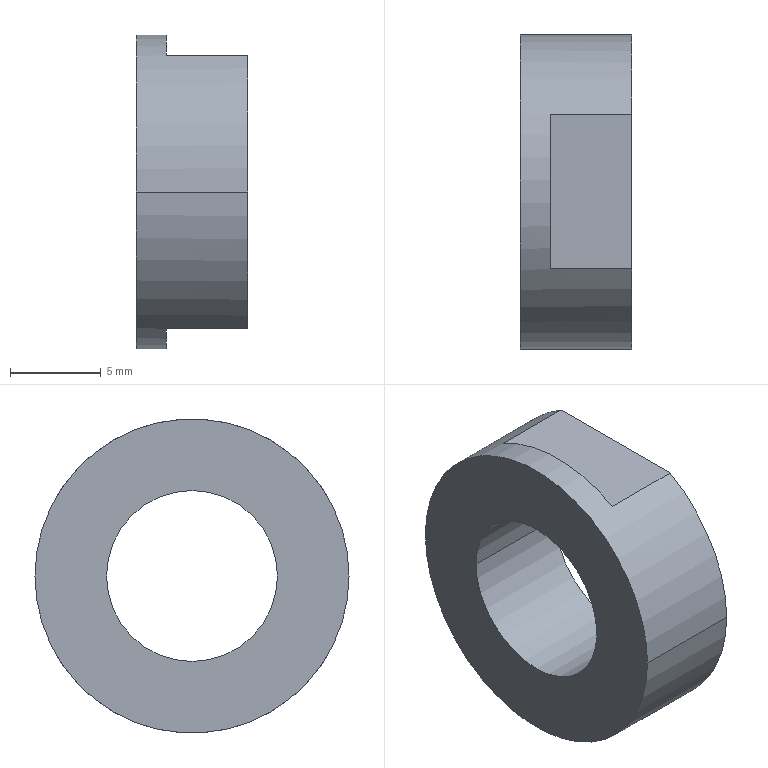Part | STEP file | BREP_4 | 1 solid | 10 faces | box 6.16 x 17.28 x 17.28 mm | volume 959.564 mm3 | plane 6 | cylinder 4 | commonest cylinder face diameters 9.4 x2 17.28 x2
STEP:
#1=CARTESIAN_POINT('',(0.,0.,0.));
#2=DIRECTION('',(0.,0.,1.));
#3=DIRECTION('',(1.,0.,0.));
#4=AXIS2_PLACEMENT_3D('',#1,#2,#3);
#5=CARTESIAN_POINT('',(56.72,-8.64,0.));
#6=VERTEX_POINT('',#5);
#7=CARTESIAN_POINT('',(56.72,8.64,0.));
#8=VERTEX_POINT('',#7);
#9=CARTESIAN_POINT('',(56.72,0.,0.));
#10=DIRECTION('',(-1.,0.,0.));
#11=DIRECTION('',(0.,-1.,0.));
#12=AXIS2_PLACEMENT_3D('',#9,#10,#11);
#13=CIRCLE('',#12,8.64);
#14=CARTESIAN_POINT('',(56.72,-8.64,8.64));
#15=DIRECTION('',(-1.,0.,0.));
#16=DIRECTION('',(0.,1.,0.));
#17=AXIS2_PLACEMENT_3D('',#14,#15,#16);
#18=PLANE('',#17);
#19=CARTESIAN_POINT('',(8.64,8.64));
#20=DIRECTION('',(-1.,0.));
#21=AXIS2_PLACEMENT_2D('',#19,#20);
#22=CIRCLE('',#21,8.64);
#23=(GEOMETRIC_REPRESENTATION_CONTEXT(2)PARAMETRIC_REPRESENTATION_CONTEXT()REPRESENTATION_CONTEXT('',''));
#24=DEFINITIONAL_REPRESENTATION('',(#22),#23);
#25=PCURVE('',#18,#24);
#26=CARTESIAN_POINT('',(59.8,0.,0.));
#27=DIRECTION('',(1.,0.,0.));
#28=DIRECTION('',(0.,1.,0.));
#29=AXIS2_PLACEMENT_3D('',#26,#27,#28);
#30=CYLINDRICAL_SURFACE('',#29,8.64);
#31=CARTESIAN_POINT('',(3.142,-3.08));
#32=DIRECTION('',(-1.,0.));
#33=VECTOR('',#32,1.);
#34=LINE('',#31,#33);
#35=(GEOMETRIC_REPRESENTATION_CONTEXT(2)PARAMETRIC_REPRESENTATION_CONTEXT()REPRESENTATION_CONTEXT('',''));
#36=DEFINITIONAL_REPRESENTATION('',(#34),#35);
#37=PCURVE('',#30,#36);
#38=SURFACE_CURVE('',#13,(#25,#37),.PCURVE_S1.);
#39=EDGE_CURVE('',#6,#8,#38,.T.);
#40=ORIENTED_EDGE('',*,*,#39,.F.);
#41=CARTESIAN_POINT('',(56.72,0.,0.));
#42=DIRECTION('',(-1.,0.,0.));
#43=DIRECTION('',(0.,1.,0.));
#44=AXIS2_PLACEMENT_3D('',#41,#42,#43);
#45=CIRCLE('',#44,8.64);
#46=CARTESIAN_POINT('',(8.64,8.64));
#47=DIRECTION('',(1.,0.));
#48=AXIS2_PLACEMENT_2D('',#46,#47);
#49=CIRCLE('',#48,8.64);
#50=(GEOMETRIC_REPRESENTATION_CONTEXT(2)PARAMETRIC_REPRESENTATION_CONTEXT()REPRESENTATION_CONTEXT('',''));
#51=DEFINITIONAL_REPRESENTATION('',(#49),#50);
#52=PCURVE('',#18,#51);
#53=CARTESIAN_POINT('',(59.8,0.,0.));
#54=DIRECTION('',(1.,0.,0.));
#55=DIRECTION('',(0.,-1.,0.));
#56=AXIS2_PLACEMENT_3D('',#53,#54,#55);
#57=CYLINDRICAL_SURFACE('',#56,8.64);
#58=CARTESIAN_POINT('',(3.142,-3.08));
#59=DIRECTION('',(-1.,0.));
#60=VECTOR('',#59,1.);
#61=LINE('',#58,#60);
#62=(GEOMETRIC_REPRESENTATION_CONTEXT(2)PARAMETRIC_REPRESENTATION_CONTEXT()REPRESENTATION_CONTEXT('',''));
#63=DEFINITIONAL_REPRESENTATION('',(#61),#62);
#64=PCURVE('',#57,#63);
#65=SURFACE_CURVE('',#45,(#52,#64),.PCURVE_S1.);
#66=EDGE_CURVE('',#8,#6,#65,.T.);
#67=ORIENTED_EDGE('',*,*,#66,.F.);
#68=EDGE_LOOP('',(#40,#67));
#69=FACE_BOUND('',#68,.F.);
#70=CARTESIAN_POINT('',(56.72,4.7,0.));
#71=VERTEX_POINT('',#70);
#72=CARTESIAN_POINT('',(56.72,-4.7,0.));
#73=VERTEX_POINT('',#72);
#74=CARTESIAN_POINT('',(56.72,0.,0.));
#75=DIRECTION('',(1.,0.,0.));
#76=DIRECTION('',(0.,1.,0.));
#77=AXIS2_PLACEMENT_3D('',#74,#75,#76);
#78=CIRCLE('',#77,4.7);
#79=CARTESIAN_POINT('',(13.34,8.64));
#80=CARTESIAN_POINT('',(13.34,0.4994));
#81=CARTESIAN_POINT('',(6.29,4.57));
#82=CARTESIAN_POINT('',(-0.76,8.64));
#83=CARTESIAN_POINT('',(6.29,12.71));
#84=CARTESIAN_POINT('',(13.34,16.781));
#85=CARTESIAN_POINT('',(13.34,8.64));
#86=(BOUNDED_CURVE()B_SPLINE_CURVE(2,(#79,#80,#81,#82,#83,#84,#85),.UNSPECIFIED.,.T.,.F.)B_SPLINE_CURVE_WITH_KNOTS((1,2,2,2,2,1),(-2.094,0.,2.094,4.189,6.283,8.378),.UNSPECIFIED.)CURVE()GEOMETRIC_REPRESENTATION_ITEM()RATIONAL_B_SPLINE_CURVE((1.,0.5,1.,0.5,1.,0.5,1.))REPRESENTATION_ITEM(''));
#87=(GEOMETRIC_REPRESENTATION_CONTEXT(2)PARAMETRIC_REPRESENTATION_CONTEXT()REPRESENTATION_CONTEXT('',''));
#88=DEFINITIONAL_REPRESENTATION('',(#86),#87);
#89=PCURVE('',#18,#88);
#90=CARTESIAN_POINT('',(59.8,0.,0.));
#91=DIRECTION('',(1.,0.,0.));
#92=DIRECTION('',(0.,-1.,0.));
#93=AXIS2_PLACEMENT_3D('',#90,#91,#92);
#94=CYLINDRICAL_SURFACE('',#93,4.7);
#95=CARTESIAN_POINT('',(3.142,-3.08));
#96=DIRECTION('',(1.,0.));
#97=VECTOR('',#96,1.);
#98=LINE('',#95,#97);
#99=(GEOMETRIC_REPRESENTATION_CONTEXT(2)PARAMETRIC_REPRESENTATION_CONTEXT()REPRESENTATION_CONTEXT('',''));
#100=DEFINITIONAL_REPRESENTATION('',(#98),#99);
#101=PCURVE('',#94,#100);
#102=SURFACE_CURVE('',#78,(#89,#101),.PCURVE_S1.);
#103=EDGE_CURVE('',#71,#73,#102,.T.);
#104=ORIENTED_EDGE('',*,*,#103,.F.);
#105=CARTESIAN_POINT('',(56.72,0.,0.));
#106=DIRECTION('',(1.,0.,0.));
#107=DIRECTION('',(0.,-1.,0.));
#108=AXIS2_PLACEMENT_3D('',#105,#106,#107);
#109=CIRCLE('',#108,4.7);
#110=CARTESIAN_POINT('',(3.94,8.64));
#111=CARTESIAN_POINT('',(3.94,16.781));
#112=CARTESIAN_POINT('',(10.99,12.71));
#113=CARTESIAN_POINT('',(18.04,8.64));
#114=CARTESIAN_POINT('',(10.99,4.57));
#115=CARTESIAN_POINT('',(3.94,0.4994));
#116=CARTESIAN_POINT('',(3.94,8.64));
#117=(BOUNDED_CURVE()B_SPLINE_CURVE(2,(#110,#111,#112,#113,#114,#115,#116),.UNSPECIFIED.,.T.,.F.)B_SPLINE_CURVE_WITH_KNOTS((1,2,2,2,2,1),(-2.094,0.,2.094,4.189,6.283,8.378),.UNSPECIFIED.)CURVE()GEOMETRIC_REPRESENTATION_ITEM()RATIONAL_B_SPLINE_CURVE((1.,0.5,1.,0.5,1.,0.5,1.))REPRESENTATION_ITEM(''));
#118=(GEOMETRIC_REPRESENTATION_CONTEXT(2)PARAMETRIC_REPRESENTATION_CONTEXT()REPRESENTATION_CONTEXT('',''));
#119=DEFINITIONAL_REPRESENTATION('',(#117),#118);
#120=PCURVE('',#18,#119);
#121=CARTESIAN_POINT('',(59.8,0.,0.));
#122=DIRECTION('',(1.,0.,0.));
#123=DIRECTION('',(0.,1.,0.));
#124=AXIS2_PLACEMENT_3D('',#121,#122,#123);
#125=CYLINDRICAL_SURFACE('',#124,4.7);
#126=CARTESIAN_POINT('',(3.142,-3.08));
#127=DIRECTION('',(1.,0.));
#128=VECTOR('',#127,1.);
#129=LINE('',#126,#128);
#130=(GEOMETRIC_REPRESENTATION_CONTEXT(2)PARAMETRIC_REPRESENTATION_CONTEXT()REPRESENTATION_CONTEXT('',''));
#131=DEFINITIONAL_REPRESENTATION('',(#129),#130);
#132=PCURVE('',#125,#131);
#133=SURFACE_CURVE('',#109,(#120,#132),.PCURVE_S1.);
#134=EDGE_CURVE('',#73,#71,#133,.T.);
#135=ORIENTED_EDGE('',*,*,#134,.F.);
#136=EDGE_LOOP('',(#104,#135));
#137=FACE_BOUND('',#136,.F.);
#138=ADVANCED_FACE('',(#69,#137),#18,.T.);
#139=CARTESIAN_POINT('',(62.88,-8.64,0.));
#140=VERTEX_POINT('',#139);
#141=CARTESIAN_POINT('',(62.88,-8.64,0.));
#142=DIRECTION('',(-1.,0.,0.));
#143=VECTOR('',#142,1.);
#144=LINE('',#141,#143);
#145=CARTESIAN_POINT('',(3.142,3.08));
#146=DIRECTION('',(0.,-1.));
#147=VECTOR('',#146,1.);
#148=LINE('',#145,#147);
#149=(GEOMETRIC_REPRESENTATION_CONTEXT(2)PARAMETRIC_REPRESENTATION_CONTEXT()REPRESENTATION_CONTEXT('',''));
#150=DEFINITIONAL_REPRESENTATION('',(#148),#149);
#151=PCURVE('',#30,#150);
#152=CARTESIAN_POINT('',(0.,3.08));
#153=DIRECTION('',(0.,-1.));
#154=VECTOR('',#153,1.);
#155=LINE('',#152,#154);
#156=(GEOMETRIC_REPRESENTATION_CONTEXT(2)PARAMETRIC_REPRESENTATION_CONTEXT()REPRESENTATION_CONTEXT('',''));
#157=DEFINITIONAL_REPRESENTATION('',(#155),#156);
#158=PCURVE('',#57,#157);
#159=SURFACE_CURVE('',#144,(#151,#158),.PCURVE_S1.);
#160=EDGE_CURVE('',#140,#6,#159,.T.);
#161=ORIENTED_EDGE('',*,*,#160,.F.);
#162=CARTESIAN_POINT('',(62.88,-4.245,7.525));
#163=VERTEX_POINT('',#162);
#164=CARTESIAN_POINT('',(62.88,0.,0.));
#165=DIRECTION('',(1.,0.,0.));
#166=DIRECTION('',(0.,-0.4914,0.8709));
#167=AXIS2_PLACEMENT_3D('',#164,#165,#166);
#168=CIRCLE('',#167,8.64);
#169=CARTESIAN_POINT('',(2.084,3.08));
#170=DIRECTION('',(1.,0.));
#171=VECTOR('',#170,1.);
#172=LINE('',#169,#171);
#173=(GEOMETRIC_REPRESENTATION_CONTEXT(2)PARAMETRIC_REPRESENTATION_CONTEXT()REPRESENTATION_CONTEXT('',''));
#174=DEFINITIONAL_REPRESENTATION('',(#172),#173);
#175=PCURVE('',#30,#174);
#176=CARTESIAN_POINT('',(62.88,-8.64,7.525));
#177=DIRECTION('',(1.,0.,0.));
#178=DIRECTION('',(0.,1.,0.));
#179=AXIS2_PLACEMENT_3D('',#176,#177,#178);
#180=PLANE('',#179);
#181=CARTESIAN_POINT('',(8.64,-7.525));
#182=DIRECTION('',(-0.4914,0.8709));
#183=AXIS2_PLACEMENT_2D('',#181,#182);
#184=CIRCLE('',#183,8.64);
#185=(GEOMETRIC_REPRESENTATION_CONTEXT(2)PARAMETRIC_REPRESENTATION_CONTEXT()REPRESENTATION_CONTEXT('',''));
#186=DEFINITIONAL_REPRESENTATION('',(#184),#185);
#187=PCURVE('',#180,#186);
#188=SURFACE_CURVE('',#168,(#175,#187),.PCURVE_S1.);
#189=EDGE_CURVE('',#163,#140,#188,.T.);
#190=ORIENTED_EDGE('',*,*,#189,.F.);
#191=CARTESIAN_POINT('',(58.38,-4.245,7.525));
#192=VERTEX_POINT('',#191);
#193=CARTESIAN_POINT('',(62.88,-4.245,7.525));
#194=DIRECTION('',(-1.,0.,0.));
#195=VECTOR('',#194,1.);
#196=LINE('',#193,#195);
#197=CARTESIAN_POINT('',(2.084,3.08));
#198=DIRECTION('',(0.,-1.));
#199=VECTOR('',#198,1.);
#200=LINE('',#197,#199);
#201=(GEOMETRIC_REPRESENTATION_CONTEXT(2)PARAMETRIC_REPRESENTATION_CONTEXT()REPRESENTATION_CONTEXT('',''));
#202=DEFINITIONAL_REPRESENTATION('',(#200),#201);
#203=PCURVE('',#30,#202);
#204=CARTESIAN_POINT('',(62.88,-4.245,7.525));
#205=DIRECTION('',(0.,0.,1.));
#206=DIRECTION('',(1.,0.,0.));
#207=AXIS2_PLACEMENT_3D('',#204,#205,#206);
#208=PLANE('',#207);
#209=CARTESIAN_POINT('',(0.,-0.000002642));
#210=DIRECTION('',(-1.,0.));
#211=VECTOR('',#210,1.);
#212=LINE('',#209,#211);
#213=(GEOMETRIC_REPRESENTATION_CONTEXT(2)PARAMETRIC_REPRESENTATION_CONTEXT()REPRESENTATION_CONTEXT('',''));
#214=DEFINITIONAL_REPRESENTATION('',(#212),#213);
#215=PCURVE('',#208,#214);
#216=SURFACE_CURVE('',#196,(#203,#215),.PCURVE_S1.);
#217=EDGE_CURVE('',#163,#192,#216,.T.);
#218=ORIENTED_EDGE('',*,*,#217,.T.);
#219=CARTESIAN_POINT('',(58.38,4.245,7.525));
#220=VERTEX_POINT('',#219);
#221=CARTESIAN_POINT('',(58.38,0.,0.));
#222=DIRECTION('',(1.,0.,0.));
#223=DIRECTION('',(0.,0.4914,0.8709));
#224=AXIS2_PLACEMENT_3D('',#221,#222,#223);
#225=CIRCLE('',#224,8.64);
#226=CARTESIAN_POINT('',(1.057,-1.42));
#227=DIRECTION('',(1.,0.));
#228=VECTOR('',#227,1.);
#229=LINE('',#226,#228);
#230=(GEOMETRIC_REPRESENTATION_CONTEXT(2)PARAMETRIC_REPRESENTATION_CONTEXT()REPRESENTATION_CONTEXT('',''));
#231=DEFINITIONAL_REPRESENTATION('',(#229),#230);
#232=PCURVE('',#30,#231);
#233=CARTESIAN_POINT('',(58.38,-4.245,8.651));
#234=DIRECTION('',(1.,0.,0.));
#235=DIRECTION('',(0.,1.,0.));
#236=AXIS2_PLACEMENT_3D('',#233,#234,#235);
#237=PLANE('',#236);
#238=CARTESIAN_POINT('',(4.245,-8.651));
#239=DIRECTION('',(0.4914,0.8709));
#240=AXIS2_PLACEMENT_2D('',#238,#239);
#241=CIRCLE('',#240,8.64);
#242=(GEOMETRIC_REPRESENTATION_CONTEXT(2)PARAMETRIC_REPRESENTATION_CONTEXT()REPRESENTATION_CONTEXT('',''));
#243=DEFINITIONAL_REPRESENTATION('',(#241),#242);
#244=PCURVE('',#237,#243);
#245=SURFACE_CURVE('',#225,(#232,#244),.PCURVE_S1.);
#246=EDGE_CURVE('',#220,#192,#245,.T.);
#247=ORIENTED_EDGE('',*,*,#246,.F.);
#248=CARTESIAN_POINT('',(62.88,4.245,7.525));
#249=VERTEX_POINT('',#248);
#250=CARTESIAN_POINT('',(58.38,4.245,7.525));
#251=DIRECTION('',(1.,0.,0.));
#252=VECTOR('',#251,1.);
#253=LINE('',#250,#252);
#254=CARTESIAN_POINT('',(1.057,-1.42));
#255=DIRECTION('',(0.,1.));
#256=VECTOR('',#255,1.);
#257=LINE('',#254,#256);
#258=(GEOMETRIC_REPRESENTATION_CONTEXT(2)PARAMETRIC_REPRESENTATION_CONTEXT()REPRESENTATION_CONTEXT('',''));
#259=DEFINITIONAL_REPRESENTATION('',(#257),#258);
#260=PCURVE('',#30,#259);
#261=CARTESIAN_POINT('',(-4.5,8.491));
#262=DIRECTION('',(1.,0.));
#263=VECTOR('',#262,1.);
#264=LINE('',#261,#263);
#265=(GEOMETRIC_REPRESENTATION_CONTEXT(2)PARAMETRIC_REPRESENTATION_CONTEXT()REPRESENTATION_CONTEXT('',''));
#266=DEFINITIONAL_REPRESENTATION('',(#264),#265);
#267=PCURVE('',#208,#266);
#268=SURFACE_CURVE('',#253,(#260,#267),.PCURVE_S1.);
#269=EDGE_CURVE('',#220,#249,#268,.T.);
#270=ORIENTED_EDGE('',*,*,#269,.T.);
#271=CARTESIAN_POINT('',(62.88,8.64,0.));
#272=VERTEX_POINT('',#271);
#273=CARTESIAN_POINT('',(62.88,0.,0.));
#274=DIRECTION('',(1.,0.,0.));
#275=DIRECTION('',(0.,1.,0.));
#276=AXIS2_PLACEMENT_3D('',#273,#274,#275);
#277=CIRCLE('',#276,8.64);
#278=CARTESIAN_POINT('',(0.,3.08));
#279=DIRECTION('',(1.,0.));
#280=VECTOR('',#279,1.);
#281=LINE('',#278,#280);
#282=(GEOMETRIC_REPRESENTATION_CONTEXT(2)PARAMETRIC_REPRESENTATION_CONTEXT()REPRESENTATION_CONTEXT('',''));
#283=DEFINITIONAL_REPRESENTATION('',(#281),#282);
#284=PCURVE('',#30,#283);
#285=CARTESIAN_POINT('',(8.64,-7.525));
#286=DIRECTION('',(1.,0.));
#287=AXIS2_PLACEMENT_2D('',#285,#286);
#288=CIRCLE('',#287,8.64);
#289=(GEOMETRIC_REPRESENTATION_CONTEXT(2)PARAMETRIC_REPRESENTATION_CONTEXT()REPRESENTATION_CONTEXT('',''));
#290=DEFINITIONAL_REPRESENTATION('',(#288),#289);
#291=PCURVE('',#180,#290);
#292=SURFACE_CURVE('',#277,(#284,#291),.PCURVE_S1.);
#293=EDGE_CURVE('',#272,#249,#292,.T.);
#294=ORIENTED_EDGE('',*,*,#293,.F.);
#295=CARTESIAN_POINT('',(62.88,8.64,0.));
#296=DIRECTION('',(-1.,0.,0.));
#297=VECTOR('',#296,1.);
#298=LINE('',#295,#297);
#299=CARTESIAN_POINT('',(0.,3.08));
#300=DIRECTION('',(0.,-1.));
#301=VECTOR('',#300,1.);
#302=LINE('',#299,#301);
#303=(GEOMETRIC_REPRESENTATION_CONTEXT(2)PARAMETRIC_REPRESENTATION_CONTEXT()REPRESENTATION_CONTEXT('',''));
#304=DEFINITIONAL_REPRESENTATION('',(#302),#303);
#305=PCURVE('',#30,#304);
#306=CARTESIAN_POINT('',(3.142,3.08));
#307=DIRECTION('',(0.,-1.));
#308=VECTOR('',#307,1.);
#309=LINE('',#306,#308);
#310=(GEOMETRIC_REPRESENTATION_CONTEXT(2)PARAMETRIC_REPRESENTATION_CONTEXT()REPRESENTATION_CONTEXT('',''));
#311=DEFINITIONAL_REPRESENTATION('',(#309),#310);
#312=PCURVE('',#57,#311);
#313=SURFACE_CURVE('',#298,(#305,#312),.PCURVE_S1.);
#314=EDGE_CURVE('',#272,#8,#313,.T.);
#315=ORIENTED_EDGE('',*,*,#314,.T.);
#316=ORIENTED_EDGE('',*,*,#39,.F.);
#317=EDGE_LOOP('',(#161,#190,#218,#247,#270,#294,#315,#316));
#318=FACE_BOUND('',#317,.T.);
#319=ADVANCED_FACE('',(#318),#30,.T.);
#320=CARTESIAN_POINT('',(62.88,4.245,-7.525));
#321=VERTEX_POINT('',#320);
#322=CARTESIAN_POINT('',(62.88,0.,0.));
#323=DIRECTION('',(1.,0.,0.));
#324=DIRECTION('',(0.,0.4914,-0.8709));
#325=AXIS2_PLACEMENT_3D('',#322,#323,#324);
#326=CIRCLE('',#325,8.64);
#327=CARTESIAN_POINT('',(2.084,3.08));
#328=DIRECTION('',(1.,0.));
#329=VECTOR('',#328,1.);
#330=LINE('',#327,#329);
#331=(GEOMETRIC_REPRESENTATION_CONTEXT(2)PARAMETRIC_REPRESENTATION_CONTEXT()REPRESENTATION_CONTEXT('',''));
#332=DEFINITIONAL_REPRESENTATION('',(#330),#331);
#333=PCURVE('',#57,#332);
#334=CARTESIAN_POINT('',(8.64,-7.525));
#335=DIRECTION('',(0.4914,-0.8709));
#336=AXIS2_PLACEMENT_2D('',#334,#335);
#337=CIRCLE('',#336,8.64);
#338=(GEOMETRIC_REPRESENTATION_CONTEXT(2)PARAMETRIC_REPRESENTATION_CONTEXT()REPRESENTATION_CONTEXT('',''));
#339=DEFINITIONAL_REPRESENTATION('',(#337),#338);
#340=PCURVE('',#180,#339);
#341=SURFACE_CURVE('',#326,(#333,#340),.PCURVE_S1.);
#342=EDGE_CURVE('',#321,#272,#341,.T.);
#343=ORIENTED_EDGE('',*,*,#342,.F.);
#344=CARTESIAN_POINT('',(58.38,4.245,-7.525));
#345=VERTEX_POINT('',#344);
#346=CARTESIAN_POINT('',(62.88,4.245,-7.525));
#347=DIRECTION('',(-1.,0.,0.));
#348=VECTOR('',#347,1.);
#349=LINE('',#346,#348);
#350=CARTESIAN_POINT('',(2.084,3.08));
#351=DIRECTION('',(0.,-1.));
#352=VECTOR('',#351,1.);
#353=LINE('',#350,#352);
#354=(GEOMETRIC_REPRESENTATION_CONTEXT(2)PARAMETRIC_REPRESENTATION_CONTEXT()REPRESENTATION_CONTEXT('',''));
#355=DEFINITIONAL_REPRESENTATION('',(#353),#354);
#356=PCURVE('',#57,#355);
#357=CARTESIAN_POINT('',(62.88,4.245,-7.525));
#358=DIRECTION('',(0.,0.,-1.));
#359=DIRECTION('',(1.,0.,0.));
#360=AXIS2_PLACEMENT_3D('',#357,#358,#359);
#361=PLANE('',#360);
#362=CARTESIAN_POINT('',(0.,-0.000002642));
#363=DIRECTION('',(-1.,0.));
#364=VECTOR('',#363,1.);
#365=LINE('',#362,#364);
#366=(GEOMETRIC_REPRESENTATION_CONTEXT(2)PARAMETRIC_REPRESENTATION_CONTEXT()REPRESENTATION_CONTEXT('',''));
#367=DEFINITIONAL_REPRESENTATION('',(#365),#366);
#368=PCURVE('',#361,#367);
#369=SURFACE_CURVE('',#349,(#356,#368),.PCURVE_S1.);
#370=EDGE_CURVE('',#321,#345,#369,.T.);
#371=ORIENTED_EDGE('',*,*,#370,.T.);
#372=CARTESIAN_POINT('',(58.38,-4.245,-7.525));
#373=VERTEX_POINT('',#372);
#374=CARTESIAN_POINT('',(58.38,0.,0.));
#375=DIRECTION('',(1.,0.,0.));
#376=DIRECTION('',(0.,-0.4914,-0.8709));
#377=AXIS2_PLACEMENT_3D('',#374,#375,#376);
#378=CIRCLE('',#377,8.64);
#379=CARTESIAN_POINT('',(-5.226,-1.42));
#380=DIRECTION('',(1.,0.));
#381=VECTOR('',#380,1.);
#382=LINE('',#379,#381);
#383=(GEOMETRIC_REPRESENTATION_CONTEXT(2)PARAMETRIC_REPRESENTATION_CONTEXT()REPRESENTATION_CONTEXT('',''));
#384=DEFINITIONAL_REPRESENTATION('',(#382),#383);
#385=PCURVE('',#57,#384);
#386=CARTESIAN_POINT('',(58.38,-4.245,-7.525));
#387=DIRECTION('',(1.,0.,0.));
#388=DIRECTION('',(0.,1.,0.));
#389=AXIS2_PLACEMENT_3D('',#386,#387,#388);
#390=PLANE('',#389);
#391=CARTESIAN_POINT('',(4.245,7.525));
#392=DIRECTION('',(-0.4914,-0.8709));
#393=AXIS2_PLACEMENT_2D('',#391,#392);
#394=CIRCLE('',#393,8.64);
#395=(GEOMETRIC_REPRESENTATION_CONTEXT(2)PARAMETRIC_REPRESENTATION_CONTEXT()REPRESENTATION_CONTEXT('',''));
#396=DEFINITIONAL_REPRESENTATION('',(#394),#395);
#397=PCURVE('',#390,#396);
#398=SURFACE_CURVE('',#378,(#385,#397),.PCURVE_S1.);
#399=EDGE_CURVE('',#373,#345,#398,.T.);
#400=ORIENTED_EDGE('',*,*,#399,.F.);
#401=CARTESIAN_POINT('',(62.88,-4.245,-7.525));
#402=VERTEX_POINT('',#401);
#403=CARTESIAN_POINT('',(58.38,-4.245,-7.525));
#404=DIRECTION('',(1.,0.,0.));
#405=VECTOR('',#404,1.);
#406=LINE('',#403,#405);
#407=CARTESIAN_POINT('',(1.057,-1.42));
#408=DIRECTION('',(0.,1.));
#409=VECTOR('',#408,1.);
#410=LINE('',#407,#409);
#411=(GEOMETRIC_REPRESENTATION_CONTEXT(2)PARAMETRIC_REPRESENTATION_CONTEXT()REPRESENTATION_CONTEXT('',''));
#412=DEFINITIONAL_REPRESENTATION('',(#410),#411);
#413=PCURVE('',#57,#412);
#414=CARTESIAN_POINT('',(-4.5,8.491));
#415=DIRECTION('',(1.,0.));
#416=VECTOR('',#415,1.);
#417=LINE('',#414,#416);
#418=(GEOMETRIC_REPRESENTATION_CONTEXT(2)PARAMETRIC_REPRESENTATION_CONTEXT()REPRESENTATION_CONTEXT('',''));
#419=DEFINITIONAL_REPRESENTATION('',(#417),#418);
#420=PCURVE('',#361,#419);
#421=SURFACE_CURVE('',#406,(#413,#420),.PCURVE_S1.);
#422=EDGE_CURVE('',#373,#402,#421,.T.);
#423=ORIENTED_EDGE('',*,*,#422,.T.);
#424=CARTESIAN_POINT('',(62.88,0.,0.));
#425=DIRECTION('',(1.,0.,0.));
#426=DIRECTION('',(0.,-1.,0.));
#427=AXIS2_PLACEMENT_3D('',#424,#425,#426);
#428=CIRCLE('',#427,8.64);
#429=CARTESIAN_POINT('',(0.,3.08));
#430=DIRECTION('',(1.,0.));
#431=VECTOR('',#430,1.);
#432=LINE('',#429,#431);
#433=(GEOMETRIC_REPRESENTATION_CONTEXT(2)PARAMETRIC_REPRESENTATION_CONTEXT()REPRESENTATION_CONTEXT('',''));
#434=DEFINITIONAL_REPRESENTATION('',(#432),#433);
#435=PCURVE('',#57,#434);
#436=CARTESIAN_POINT('',(8.64,-7.525));
#437=DIRECTION('',(-1.,0.));
#438=AXIS2_PLACEMENT_2D('',#436,#437);
#439=CIRCLE('',#438,8.64);
#440=(GEOMETRIC_REPRESENTATION_CONTEXT(2)PARAMETRIC_REPRESENTATION_CONTEXT()REPRESENTATION_CONTEXT('',''));
#441=DEFINITIONAL_REPRESENTATION('',(#439),#440);
#442=PCURVE('',#180,#441);
#443=SURFACE_CURVE('',#428,(#435,#442),.PCURVE_S1.);
#444=EDGE_CURVE('',#140,#402,#443,.T.);
#445=ORIENTED_EDGE('',*,*,#444,.F.);
#446=ORIENTED_EDGE('',*,*,#160,.T.);
#447=ORIENTED_EDGE('',*,*,#66,.F.);
#448=ORIENTED_EDGE('',*,*,#314,.F.);
#449=EDGE_LOOP('',(#343,#371,#400,#423,#445,#446,#447,#448));
#450=FACE_BOUND('',#449,.T.);
#451=ADVANCED_FACE('',(#450),#57,.T.);
#452=CARTESIAN_POINT('',(62.88,4.245,-7.525));
#453=DIRECTION('',(0.,-1.,0.));
#454=VECTOR('',#453,1.);
#455=LINE('',#452,#454);
#456=CARTESIAN_POINT('',(12.885,-15.05));
#457=DIRECTION('',(-1.,0.));
#458=VECTOR('',#457,1.);
#459=LINE('',#456,#458);
#460=(GEOMETRIC_REPRESENTATION_CONTEXT(2)PARAMETRIC_REPRESENTATION_CONTEXT()REPRESENTATION_CONTEXT('',''));
#461=DEFINITIONAL_REPRESENTATION('',(#459),#460);
#462=PCURVE('',#180,#461);
#463=CARTESIAN_POINT('',(0.,-0.000002642));
#464=DIRECTION('',(0.,1.));
#465=VECTOR('',#464,1.);
#466=LINE('',#463,#465);
#467=(GEOMETRIC_REPRESENTATION_CONTEXT(2)PARAMETRIC_REPRESENTATION_CONTEXT()REPRESENTATION_CONTEXT('',''));
#468=DEFINITIONAL_REPRESENTATION('',(#466),#467);
#469=PCURVE('',#361,#468);
#470=SURFACE_CURVE('',#455,(#462,#469),.PCURVE_S1.);
#471=EDGE_CURVE('',#321,#402,#470,.T.);
#472=ORIENTED_EDGE('',*,*,#471,.T.);
#473=ORIENTED_EDGE('',*,*,#444,.F.);
#474=ORIENTED_EDGE('',*,*,#189,.F.);
#475=CARTESIAN_POINT('',(62.88,-4.245,7.525));
#476=DIRECTION('',(0.,1.,0.));
#477=VECTOR('',#476,1.);
#478=LINE('',#475,#477);
#479=CARTESIAN_POINT('',(4.395,-0.000001491));
#480=DIRECTION('',(1.,0.));
#481=VECTOR('',#480,1.);
#482=LINE('',#479,#481);
#483=(GEOMETRIC_REPRESENTATION_CONTEXT(2)PARAMETRIC_REPRESENTATION_CONTEXT()REPRESENTATION_CONTEXT('',''));
#484=DEFINITIONAL_REPRESENTATION('',(#482),#483);
#485=PCURVE('',#180,#484);
#486=CARTESIAN_POINT('',(0.,-0.000002642));
#487=DIRECTION('',(0.,1.));
#488=VECTOR('',#487,1.);
#489=LINE('',#486,#488);
#490=(GEOMETRIC_REPRESENTATION_CONTEXT(2)PARAMETRIC_REPRESENTATION_CONTEXT()REPRESENTATION_CONTEXT('',''));
#491=DEFINITIONAL_REPRESENTATION('',(#489),#490);
#492=PCURVE('',#208,#491);
#493=SURFACE_CURVE('',#478,(#485,#492),.PCURVE_S1.);
#494=EDGE_CURVE('',#163,#249,#493,.T.);
#495=ORIENTED_EDGE('',*,*,#494,.T.);
#496=ORIENTED_EDGE('',*,*,#293,.F.);
#497=ORIENTED_EDGE('',*,*,#342,.F.);
#498=EDGE_LOOP('',(#472,#473,#474,#495,#496,#497));
#499=FACE_BOUND('',#498,.F.);
#500=CARTESIAN_POINT('',(62.88,4.7,0.));
#501=VERTEX_POINT('',#500);
#502=CARTESIAN_POINT('',(62.88,-4.7,0.));
#503=VERTEX_POINT('',#502);
#504=CARTESIAN_POINT('',(62.88,0.,0.));
#505=DIRECTION('',(-1.,0.,0.));
#506=DIRECTION('',(0.,1.,0.));
#507=AXIS2_PLACEMENT_3D('',#504,#505,#506);
#508=CIRCLE('',#507,4.7);
#509=CARTESIAN_POINT('',(13.34,-7.525));
#510=CARTESIAN_POINT('',(13.34,-15.666));
#511=CARTESIAN_POINT('',(6.29,-11.595));
#512=CARTESIAN_POINT('',(-0.76,-7.525));
#513=CARTESIAN_POINT('',(6.29,-3.455));
#514=CARTESIAN_POINT('',(13.34,0.6156));
#515=CARTESIAN_POINT('',(13.34,-7.525));
#516=(BOUNDED_CURVE()B_SPLINE_CURVE(2,(#509,#510,#511,#512,#513,#514,#515),.UNSPECIFIED.,.T.,.F.)B_SPLINE_CURVE_WITH_KNOTS((1,2,2,2,2,1),(-2.094,0.,2.094,4.189,6.283,8.378),.UNSPECIFIED.)CURVE()GEOMETRIC_REPRESENTATION_ITEM()RATIONAL_B_SPLINE_CURVE((1.,0.5,1.,0.5,1.,0.5,1.))REPRESENTATION_ITEM(''));
#517=(GEOMETRIC_REPRESENTATION_CONTEXT(2)PARAMETRIC_REPRESENTATION_CONTEXT()REPRESENTATION_CONTEXT('',''));
#518=DEFINITIONAL_REPRESENTATION('',(#516),#517);
#519=PCURVE('',#180,#518);
#520=CARTESIAN_POINT('',(6.283,3.08));
#521=DIRECTION('',(-1.,0.));
#522=VECTOR('',#521,1.);
#523=LINE('',#520,#522);
#524=(GEOMETRIC_REPRESENTATION_CONTEXT(2)PARAMETRIC_REPRESENTATION_CONTEXT()REPRESENTATION_CONTEXT('',''));
#525=DEFINITIONAL_REPRESENTATION('',(#523),#524);
#526=PCURVE('',#125,#525);
#527=SURFACE_CURVE('',#508,(#519,#526),.PCURVE_S1.);
#528=EDGE_CURVE('',#501,#503,#527,.T.);
#529=ORIENTED_EDGE('',*,*,#528,.F.);
#530=CARTESIAN_POINT('',(62.88,0.,0.));
#531=DIRECTION('',(-1.,0.,0.));
#532=DIRECTION('',(0.,-1.,0.));
#533=AXIS2_PLACEMENT_3D('',#530,#531,#532);
#534=CIRCLE('',#533,4.7);
#535=CARTESIAN_POINT('',(3.94,-7.525));
#536=CARTESIAN_POINT('',(3.94,0.6156));
#537=CARTESIAN_POINT('',(10.99,-3.455));
#538=CARTESIAN_POINT('',(18.04,-7.525));
#539=CARTESIAN_POINT('',(10.99,-11.595));
#540=CARTESIAN_POINT('',(3.94,-15.666));
#541=CARTESIAN_POINT('',(3.94,-7.525));
#542=(BOUNDED_CURVE()B_SPLINE_CURVE(2,(#535,#536,#537,#538,#539,#540,#541),.UNSPECIFIED.,.T.,.F.)B_SPLINE_CURVE_WITH_KNOTS((1,2,2,2,2,1),(-2.094,0.,2.094,4.189,6.283,8.378),.UNSPECIFIED.)CURVE()GEOMETRIC_REPRESENTATION_ITEM()RATIONAL_B_SPLINE_CURVE((1.,0.5,1.,0.5,1.,0.5,1.))REPRESENTATION_ITEM(''));
#543=(GEOMETRIC_REPRESENTATION_CONTEXT(2)PARAMETRIC_REPRESENTATION_CONTEXT()REPRESENTATION_CONTEXT('',''));
#544=DEFINITIONAL_REPRESENTATION('',(#542),#543);
#545=PCURVE('',#180,#544);
#546=CARTESIAN_POINT('',(6.283,3.08));
#547=DIRECTION('',(-1.,0.));
#548=VECTOR('',#547,1.);
#549=LINE('',#546,#548);
#550=(GEOMETRIC_REPRESENTATION_CONTEXT(2)PARAMETRIC_REPRESENTATION_CONTEXT()REPRESENTATION_CONTEXT('',''));
#551=DEFINITIONAL_REPRESENTATION('',(#549),#550);
#552=PCURVE('',#94,#551);
#553=SURFACE_CURVE('',#534,(#545,#552),.PCURVE_S1.);
#554=EDGE_CURVE('',#503,#501,#553,.T.);
#555=ORIENTED_EDGE('',*,*,#554,.F.);
#556=EDGE_LOOP('',(#529,#555));
#557=FACE_BOUND('',#556,.F.);
#558=ADVANCED_FACE('',(#499,#557),#180,.T.);
#559=ORIENTED_EDGE('',*,*,#370,.F.);
#560=ORIENTED_EDGE('',*,*,#471,.T.);
#561=ORIENTED_EDGE('',*,*,#422,.F.);
#562=CARTESIAN_POINT('',(58.38,4.245,-7.525));
#563=DIRECTION('',(0.,-1.,0.));
#564=VECTOR('',#563,1.);
#565=LINE('',#562,#564);
#566=CARTESIAN_POINT('',(-4.5,-0.000002642));
#567=DIRECTION('',(0.,1.));
#568=VECTOR('',#567,1.);
#569=LINE('',#566,#568);
#570=(GEOMETRIC_REPRESENTATION_CONTEXT(2)PARAMETRIC_REPRESENTATION_CONTEXT()REPRESENTATION_CONTEXT('',''));
#571=DEFINITIONAL_REPRESENTATION('',(#569),#570);
#572=PCURVE('',#361,#571);
#573=CARTESIAN_POINT('',(8.491,0.000001491));
#574=DIRECTION('',(-1.,0.));
#575=VECTOR('',#574,1.);
#576=LINE('',#573,#575);
#577=(GEOMETRIC_REPRESENTATION_CONTEXT(2)PARAMETRIC_REPRESENTATION_CONTEXT()REPRESENTATION_CONTEXT('',''));
#578=DEFINITIONAL_REPRESENTATION('',(#576),#577);
#579=PCURVE('',#390,#578);
#580=SURFACE_CURVE('',#565,(#572,#579),.PCURVE_S1.);
#581=EDGE_CURVE('',#345,#373,#580,.T.);
#582=ORIENTED_EDGE('',*,*,#581,.F.);
#583=EDGE_LOOP('',(#559,#560,#561,#582));
#584=FACE_BOUND('',#583,.T.);
#585=ADVANCED_FACE('',(#584),#361,.T.);
#586=ORIENTED_EDGE('',*,*,#399,.F.);
#587=ORIENTED_EDGE('',*,*,#581,.F.);
#588=EDGE_LOOP('',(#586,#587));
#589=FACE_BOUND('',#588,.F.);
#590=ADVANCED_FACE('',(#589),#390,.T.);
#591=ORIENTED_EDGE('',*,*,#269,.F.);
#592=CARTESIAN_POINT('',(58.38,-4.245,7.525));
#593=DIRECTION('',(0.,1.,0.));
#594=VECTOR('',#593,1.);
#595=LINE('',#592,#594);
#596=CARTESIAN_POINT('',(-4.5,-0.000002642));
#597=DIRECTION('',(0.,1.));
#598=VECTOR('',#597,1.);
#599=LINE('',#596,#598);
#600=(GEOMETRIC_REPRESENTATION_CONTEXT(2)PARAMETRIC_REPRESENTATION_CONTEXT()REPRESENTATION_CONTEXT('',''));
#601=DEFINITIONAL_REPRESENTATION('',(#599),#600);
#602=PCURVE('',#208,#601);
#603=CARTESIAN_POINT('',(-0.000002642,-1.126));
#604=DIRECTION('',(1.,0.));
#605=VECTOR('',#604,1.);
#606=LINE('',#603,#605);
#607=(GEOMETRIC_REPRESENTATION_CONTEXT(2)PARAMETRIC_REPRESENTATION_CONTEXT()REPRESENTATION_CONTEXT('',''));
#608=DEFINITIONAL_REPRESENTATION('',(#606),#607);
#609=PCURVE('',#237,#608);
#610=SURFACE_CURVE('',#595,(#602,#609),.PCURVE_S1.);
#611=EDGE_CURVE('',#192,#220,#610,.T.);
#612=ORIENTED_EDGE('',*,*,#611,.F.);
#613=ORIENTED_EDGE('',*,*,#217,.F.);
#614=ORIENTED_EDGE('',*,*,#494,.T.);
#615=EDGE_LOOP('',(#591,#612,#613,#614));
#616=FACE_BOUND('',#615,.T.);
#617=ADVANCED_FACE('',(#616),#208,.T.);
#618=ORIENTED_EDGE('',*,*,#246,.F.);
#619=ORIENTED_EDGE('',*,*,#611,.F.);
#620=EDGE_LOOP('',(#618,#619));
#621=FACE_BOUND('',#620,.F.);
#622=ADVANCED_FACE('',(#621),#237,.T.);
#623=CARTESIAN_POINT('',(62.88,-4.7,0.));
#624=DIRECTION('',(-1.,0.,0.));
#625=VECTOR('',#624,1.);
#626=LINE('',#623,#625);
#627=CARTESIAN_POINT('',(3.142,3.08));
#628=DIRECTION('',(0.,-1.));
#629=VECTOR('',#628,1.);
#630=LINE('',#627,#629);
#631=(GEOMETRIC_REPRESENTATION_CONTEXT(2)PARAMETRIC_REPRESENTATION_CONTEXT()REPRESENTATION_CONTEXT('',''));
#632=DEFINITIONAL_REPRESENTATION('',(#630),#631);
#633=PCURVE('',#125,#632);
#634=CARTESIAN_POINT('',(6.283,3.08));
#635=DIRECTION('',(0.,-1.));
#636=VECTOR('',#635,1.);
#637=LINE('',#634,#636);
#638=(GEOMETRIC_REPRESENTATION_CONTEXT(2)PARAMETRIC_REPRESENTATION_CONTEXT()REPRESENTATION_CONTEXT('',''));
#639=DEFINITIONAL_REPRESENTATION('',(#637),#638);
#640=PCURVE('',#94,#639);
#641=SURFACE_CURVE('',#626,(#633,#640),.PCURVE_S1.);
#642=EDGE_CURVE('',#503,#73,#641,.T.);
#643=ORIENTED_EDGE('',*,*,#642,.T.);
#644=ORIENTED_EDGE('',*,*,#134,.T.);
#645=CARTESIAN_POINT('',(62.88,4.7,0.));
#646=DIRECTION('',(-1.,0.,0.));
#647=VECTOR('',#646,1.);
#648=LINE('',#645,#647);
#649=CARTESIAN_POINT('',(6.283,3.08));
#650=DIRECTION('',(0.,-1.));
#651=VECTOR('',#650,1.);
#652=LINE('',#649,#651);
#653=(GEOMETRIC_REPRESENTATION_CONTEXT(2)PARAMETRIC_REPRESENTATION_CONTEXT()REPRESENTATION_CONTEXT('',''));
#654=DEFINITIONAL_REPRESENTATION('',(#652),#653);
#655=PCURVE('',#125,#654);
#656=CARTESIAN_POINT('',(3.142,3.08));
#657=DIRECTION('',(0.,-1.));
#658=VECTOR('',#657,1.);
#659=LINE('',#656,#658);
#660=(GEOMETRIC_REPRESENTATION_CONTEXT(2)PARAMETRIC_REPRESENTATION_CONTEXT()REPRESENTATION_CONTEXT('',''));
#661=DEFINITIONAL_REPRESENTATION('',(#659),#660);
#662=PCURVE('',#94,#661);
#663=SURFACE_CURVE('',#648,(#655,#662),.PCURVE_S1.);
#664=EDGE_CURVE('',#501,#71,#663,.T.);
#665=ORIENTED_EDGE('',*,*,#664,.F.);
#666=ORIENTED_EDGE('',*,*,#528,.T.);
#667=EDGE_LOOP('',(#643,#644,#665,#666));
#668=FACE_BOUND('',#667,.F.);
#669=ADVANCED_FACE('',(#668),#125,.F.);
#670=ORIENTED_EDGE('',*,*,#103,.T.);
#671=ORIENTED_EDGE('',*,*,#642,.F.);
#672=ORIENTED_EDGE('',*,*,#554,.T.);
#673=ORIENTED_EDGE('',*,*,#664,.T.);
#674=EDGE_LOOP('',(#670,#671,#672,#673));
#675=FACE_BOUND('',#674,.F.);
#676=ADVANCED_FACE('',(#675),#94,.F.);
#677=CLOSED_SHELL('',(#138,#319,#451,#558,#585,#590,#617,#622,#669,#676));
#678=MANIFOLD_SOLID_BREP('',#677);
#679=(LENGTH_UNIT()NAMED_UNIT(*)SI_UNIT(.MILLI.,.METRE.));
#680=UNCERTAINTY_MEASURE_WITH_UNIT(LENGTH_MEASURE(0.000001),#679,'','');
#681=(NAMED_UNIT(*)PLANE_ANGLE_UNIT()SI_UNIT($,.RADIAN.));
#682=(NAMED_UNIT(*)SI_UNIT($,.STERADIAN.)SOLID_ANGLE_UNIT());
#683=(GEOMETRIC_REPRESENTATION_CONTEXT(3)GLOBAL_UNCERTAINTY_ASSIGNED_CONTEXT((#680))GLOBAL_UNIT_ASSIGNED_CONTEXT((#679,#681,#682))REPRESENTATION_CONTEXT('',''));
#684=ADVANCED_BREP_SHAPE_REPRESENTATION('',(#4,#678),#683);